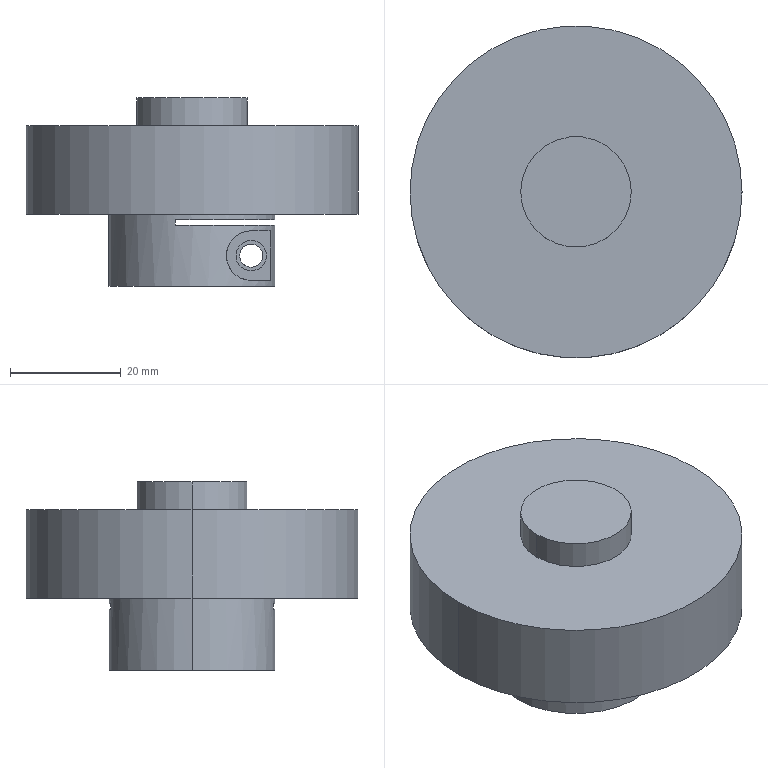Part | STEP file | B-PRF60 bottom cover plate_D6-60 D7-14 standard | 1 solid | 60 faces | box 60 x 60 x 34 mm | volume 41356 mm3 | cylinder 29 | plane 23 | cone 8 | commonest cylinder face diameters 3.3 x8 14 x3 14.5 x3 4.2 x2 5.5 x2 20 x2